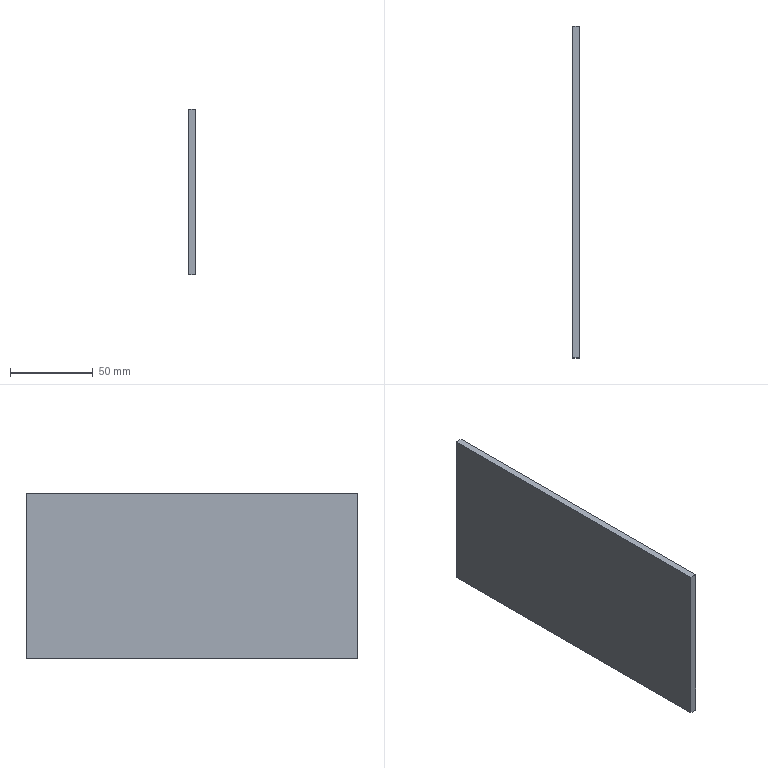Part | SolidWorks | features Extrusion 1 | 1 solid | 6 faces | box 4 x 200 x 100 mm | volume 80000 mm3 | plane 6
STEP:
#1=CARTESIAN_POINT('',(0.,200.,0.));
#2=VERTEX_POINT('',#1);
#3=CARTESIAN_POINT('',(0.,0.,0.));
#4=VERTEX_POINT('',#3);
#5=CARTESIAN_POINT('',(0.,0.,0.));
#6=DIRECTION('',(0.,-1.,0.));
#7=VECTOR('',#6,1000.);
#8=LINE('',#5,#7);
#9=EDGE_CURVE('',#2,#4,#8,.T.);
#10=ORIENTED_EDGE('',*,*,#9,.T.);
#11=CARTESIAN_POINT('',(4.,0.,0.));
#12=VERTEX_POINT('',#11);
#13=CARTESIAN_POINT('',(4.,0.,0.));
#14=DIRECTION('',(-1.,0.,0.));
#15=VECTOR('',#14,1000.);
#16=LINE('',#13,#15);
#17=EDGE_CURVE('',#12,#4,#16,.T.);
#18=ORIENTED_EDGE('',*,*,#17,.F.);
#19=CARTESIAN_POINT('',(4.,200.,0.));
#20=VERTEX_POINT('',#19);
#21=CARTESIAN_POINT('',(4.,0.,0.));
#22=DIRECTION('',(0.,-1.,0.));
#23=VECTOR('',#22,1000.);
#24=LINE('',#21,#23);
#25=EDGE_CURVE('',#20,#12,#24,.T.);
#26=ORIENTED_EDGE('',*,*,#25,.F.);
#27=CARTESIAN_POINT('',(4.,200.,0.));
#28=DIRECTION('',(-1.,0.,0.));
#29=VECTOR('',#28,1000.);
#30=LINE('',#27,#29);
#31=EDGE_CURVE('',#20,#2,#30,.T.);
#32=ORIENTED_EDGE('',*,*,#31,.T.);
#33=EDGE_LOOP('',(#10,#18,#26,#32));
#34=FACE_OUTER_BOUND('',#33,.T.);
#35=CARTESIAN_POINT('',(4.,0.,0.));
#36=DIRECTION('',(0.,0.,-1.));
#37=DIRECTION('',(-1.,0.,0.));
#38=AXIS2_PLACEMENT_3D('',#35,#36,#37);
#39=PLANE('',#38);
#40=ADVANCED_FACE('',(#34),#39,.F.);
#41=CARTESIAN_POINT('',(0.,0.,-100.));
#42=VERTEX_POINT('',#41);
#43=CARTESIAN_POINT('',(0.,0.,0.));
#44=DIRECTION('',(0.,0.,-1.));
#45=VECTOR('',#44,1000.);
#46=LINE('',#43,#45);
#47=EDGE_CURVE('',#4,#42,#46,.T.);
#48=ORIENTED_EDGE('',*,*,#47,.T.);
#49=CARTESIAN_POINT('',(4.,0.,-100.));
#50=VERTEX_POINT('',#49);
#51=CARTESIAN_POINT('',(4.,0.,-100.));
#52=DIRECTION('',(-1.,0.,0.));
#53=VECTOR('',#52,1000.);
#54=LINE('',#51,#53);
#55=EDGE_CURVE('',#50,#42,#54,.T.);
#56=ORIENTED_EDGE('',*,*,#55,.F.);
#57=CARTESIAN_POINT('',(4.,0.,0.));
#58=DIRECTION('',(0.,0.,-1.));
#59=VECTOR('',#58,1000.);
#60=LINE('',#57,#59);
#61=EDGE_CURVE('',#12,#50,#60,.T.);
#62=ORIENTED_EDGE('',*,*,#61,.F.);
#63=ORIENTED_EDGE('',*,*,#17,.T.);
#64=EDGE_LOOP('',(#48,#56,#62,#63));
#65=FACE_OUTER_BOUND('',#64,.T.);
#66=CARTESIAN_POINT('',(4.,0.,0.));
#67=DIRECTION('',(0.,1.,0.));
#68=DIRECTION('',(0.,0.,1.));
#69=AXIS2_PLACEMENT_3D('',#66,#67,#68);
#70=PLANE('',#69);
#71=ADVANCED_FACE('',(#65),#70,.F.);
#72=CARTESIAN_POINT('',(0.,200.,-100.));
#73=VERTEX_POINT('',#72);
#74=CARTESIAN_POINT('',(0.,0.,-100.));
#75=DIRECTION('',(0.,1.,0.));
#76=VECTOR('',#75,1000.);
#77=LINE('',#74,#76);
#78=EDGE_CURVE('',#42,#73,#77,.T.);
#79=ORIENTED_EDGE('',*,*,#78,.T.);
#80=CARTESIAN_POINT('',(4.,200.,-100.));
#81=VERTEX_POINT('',#80);
#82=CARTESIAN_POINT('',(4.,200.,-100.));
#83=DIRECTION('',(-1.,0.,0.));
#84=VECTOR('',#83,1000.);
#85=LINE('',#82,#84);
#86=EDGE_CURVE('',#81,#73,#85,.T.);
#87=ORIENTED_EDGE('',*,*,#86,.F.);
#88=CARTESIAN_POINT('',(4.,0.,-100.));
#89=DIRECTION('',(0.,1.,0.));
#90=VECTOR('',#89,1000.);
#91=LINE('',#88,#90);
#92=EDGE_CURVE('',#50,#81,#91,.T.);
#93=ORIENTED_EDGE('',*,*,#92,.F.);
#94=ORIENTED_EDGE('',*,*,#55,.T.);
#95=EDGE_LOOP('',(#79,#87,#93,#94));
#96=FACE_OUTER_BOUND('',#95,.T.);
#97=CARTESIAN_POINT('',(4.,0.,-100.));
#98=DIRECTION('',(0.,0.,1.));
#99=DIRECTION('',(1.,0.,0.));
#100=AXIS2_PLACEMENT_3D('',#97,#98,#99);
#101=PLANE('',#100);
#102=ADVANCED_FACE('',(#96),#101,.F.);
#103=CARTESIAN_POINT('',(0.,200.,0.));
#104=DIRECTION('',(0.,0.,1.));
#105=VECTOR('',#104,1000.);
#106=LINE('',#103,#105);
#107=EDGE_CURVE('',#73,#2,#106,.T.);
#108=ORIENTED_EDGE('',*,*,#107,.T.);
#109=ORIENTED_EDGE('',*,*,#31,.F.);
#110=CARTESIAN_POINT('',(4.,200.,0.));
#111=DIRECTION('',(0.,0.,1.));
#112=VECTOR('',#111,1000.);
#113=LINE('',#110,#112);
#114=EDGE_CURVE('',#81,#20,#113,.T.);
#115=ORIENTED_EDGE('',*,*,#114,.F.);
#116=ORIENTED_EDGE('',*,*,#86,.T.);
#117=EDGE_LOOP('',(#108,#109,#115,#116));
#118=FACE_OUTER_BOUND('',#117,.T.);
#119=CARTESIAN_POINT('',(4.,200.,0.));
#120=DIRECTION('',(0.,-1.,0.));
#121=DIRECTION('',(0.,0.,-1.));
#122=AXIS2_PLACEMENT_3D('',#119,#120,#121);
#123=PLANE('',#122);
#124=ADVANCED_FACE('',(#118),#123,.F.);
#125=ORIENTED_EDGE('',*,*,#25,.T.);
#126=ORIENTED_EDGE('',*,*,#61,.T.);
#127=ORIENTED_EDGE('',*,*,#92,.T.);
#128=ORIENTED_EDGE('',*,*,#114,.T.);
#129=EDGE_LOOP('',(#125,#126,#127,#128));
#130=FACE_OUTER_BOUND('',#129,.T.);
#131=CARTESIAN_POINT('',(4.,0.,0.));
#132=DIRECTION('',(-1.,0.,0.));
#133=DIRECTION('',(0.,0.,1.));
#134=AXIS2_PLACEMENT_3D('',#131,#132,#133);
#135=PLANE('',#134);
#136=ADVANCED_FACE('',(#130),#135,.F.);
#137=ORIENTED_EDGE('',*,*,#9,.F.);
#138=ORIENTED_EDGE('',*,*,#107,.F.);
#139=ORIENTED_EDGE('',*,*,#78,.F.);
#140=ORIENTED_EDGE('',*,*,#47,.F.);
#141=EDGE_LOOP('',(#137,#138,#139,#140));
#142=FACE_OUTER_BOUND('',#141,.T.);
#143=CARTESIAN_POINT('',(0.,0.,0.));
#144=DIRECTION('',(-1.,0.,0.));
#145=DIRECTION('',(0.,0.,1.));
#146=AXIS2_PLACEMENT_3D('',#143,#144,#145);
#147=PLANE('',#146);
#148=ADVANCED_FACE('',(#142),#147,.T.);
#149=CLOSED_SHELL('',(#40,#71,#102,#124,#136,#148));
#150=MANIFOLD_SOLID_BREP('',#149);
#151=CARTESIAN_POINT('',(0.,0.,0.));
#152=DIRECTION('',(0.,0.,1.));
#153=DIRECTION('',(1.,0.,0.));
#154=AXIS2_PLACEMENT_3D('',#151,#152,#153);
#155=(LENGTH_UNIT()NAMED_UNIT(*)SI_UNIT(.MILLI.,.METRE.));
#156=UNCERTAINTY_MEASURE_WITH_UNIT(LENGTH_MEASURE(0.00001),#155,'','');
#157=(NAMED_UNIT(*)PLANE_ANGLE_UNIT()SI_UNIT($,.RADIAN.));
#158=(NAMED_UNIT(*)SI_UNIT($,.STERADIAN.)SOLID_ANGLE_UNIT());
#159=(GEOMETRIC_REPRESENTATION_CONTEXT(3)GLOBAL_UNCERTAINTY_ASSIGNED_CONTEXT((#156))GLOBAL_UNIT_ASSIGNED_CONTEXT((#155,#157,#158))REPRESENTATION_CONTEXT('',''));
#160=ADVANCED_BREP_SHAPE_REPRESENTATION('',(#150,#154),#159);